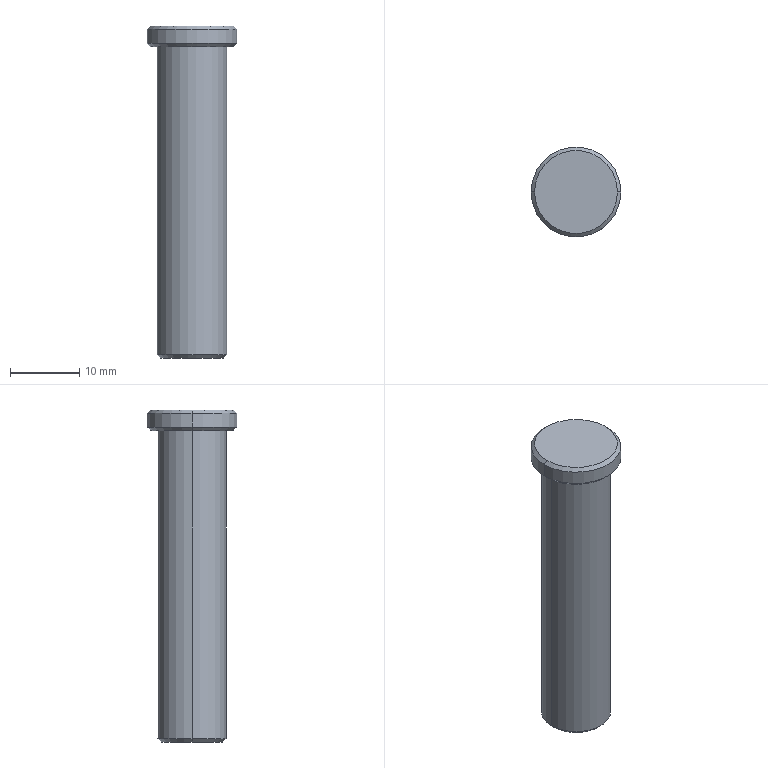Part | SolidWorks | features Chamfer 1, Extrusion 1, ICE 1 | 1 solid | 13 faces | box 13 x 13 x 48 mm | volume 3919 mm3 | cone 6 | cylinder 4 | plane 3 | commonest cylinder face diameters 10 x2 13 x2
STEP:
#1=CARTESIAN_POINT('',(-4.5,0.,0.));
#2=VERTEX_POINT('',#1);
#3=CARTESIAN_POINT('',(4.5,0.,0.));
#4=VERTEX_POINT('',#3);
#5=CARTESIAN_POINT('',(0.,0.,0.));
#6=DIRECTION('',(0.,0.,-1.));
#7=DIRECTION('',(1.,0.,0.));
#8=AXIS2_PLACEMENT_3D('',#5,#6,#7);
#9=CIRCLE('',#8,4.5);
#10=EDGE_CURVE('',#2,#4,#9,.T.);
#11=ORIENTED_EDGE('',*,*,#10,.F.);
#12=CARTESIAN_POINT('',(-5.,0.,0.5));
#13=VERTEX_POINT('',#12);
#14=CARTESIAN_POINT('',(-5.,0.,0.5));
#15=DIRECTION('',(-0.7071,0.,0.7071));
#16=VECTOR('',#15,1000.);
#17=LINE('',#14,#16);
#18=EDGE_CURVE('',#2,#13,#17,.T.);
#19=ORIENTED_EDGE('',*,*,#18,.T.);
#20=CARTESIAN_POINT('',(5.,0.,0.5));
#21=VERTEX_POINT('',#20);
#22=CARTESIAN_POINT('',(0.,0.,0.5));
#23=DIRECTION('',(0.,0.,1.));
#24=DIRECTION('',(1.,0.,0.));
#25=AXIS2_PLACEMENT_3D('',#22,#23,#24);
#26=CIRCLE('',#25,5.);
#27=EDGE_CURVE('',#21,#13,#26,.T.);
#28=ORIENTED_EDGE('',*,*,#27,.F.);
#29=CARTESIAN_POINT('',(5.,0.,0.5));
#30=DIRECTION('',(0.7071,0.,0.7071));
#31=VECTOR('',#30,1000.);
#32=LINE('',#29,#31);
#33=EDGE_CURVE('',#4,#21,#32,.T.);
#34=ORIENTED_EDGE('',*,*,#33,.F.);
#35=EDGE_LOOP('',(#11,#19,#28,#34));
#36=FACE_OUTER_BOUND('',#35,.T.);
#37=CARTESIAN_POINT('',(0.,0.,0.5));
#38=DIRECTION('',(0.,0.,1.));
#39=DIRECTION('',(1.,0.,0.));
#40=AXIS2_PLACEMENT_3D('',#37,#38,#39);
#41=CONICAL_SURFACE('',#40,5.,0.7854);
#42=ADVANCED_FACE('',(#36),#41,.T.);
#43=CARTESIAN_POINT('',(-6.,0.,45.));
#44=VERTEX_POINT('',#43);
#45=CARTESIAN_POINT('',(6.,0.,45.));
#46=VERTEX_POINT('',#45);
#47=CARTESIAN_POINT('',(0.,0.,45.));
#48=DIRECTION('',(0.,0.,-1.));
#49=DIRECTION('',(1.,0.,0.));
#50=AXIS2_PLACEMENT_3D('',#47,#48,#49);
#51=CIRCLE('',#50,6.);
#52=EDGE_CURVE('',#44,#46,#51,.T.);
#53=ORIENTED_EDGE('',*,*,#52,.F.);
#54=CARTESIAN_POINT('',(-6.5,0.,45.5));
#55=VERTEX_POINT('',#54);
#56=CARTESIAN_POINT('',(-6.5,0.,45.5));
#57=DIRECTION('',(-0.7071,0.,0.7071));
#58=VECTOR('',#57,1000.);
#59=LINE('',#56,#58);
#60=EDGE_CURVE('',#44,#55,#59,.T.);
#61=ORIENTED_EDGE('',*,*,#60,.T.);
#62=CARTESIAN_POINT('',(6.5,0.,45.5));
#63=VERTEX_POINT('',#62);
#64=CARTESIAN_POINT('',(0.,0.,45.5));
#65=DIRECTION('',(0.,0.,1.));
#66=DIRECTION('',(1.,0.,0.));
#67=AXIS2_PLACEMENT_3D('',#64,#65,#66);
#68=CIRCLE('',#67,6.5);
#69=EDGE_CURVE('',#63,#55,#68,.T.);
#70=ORIENTED_EDGE('',*,*,#69,.F.);
#71=CARTESIAN_POINT('',(6.5,0.,45.5));
#72=DIRECTION('',(0.7071,0.,0.7071));
#73=VECTOR('',#72,1000.);
#74=LINE('',#71,#73);
#75=EDGE_CURVE('',#46,#63,#74,.T.);
#76=ORIENTED_EDGE('',*,*,#75,.F.);
#77=EDGE_LOOP('',(#53,#61,#70,#76));
#78=FACE_OUTER_BOUND('',#77,.T.);
#79=CARTESIAN_POINT('',(0.,0.,45.5));
#80=DIRECTION('',(0.,0.,1.));
#81=DIRECTION('',(1.,0.,0.));
#82=AXIS2_PLACEMENT_3D('',#79,#80,#81);
#83=CONICAL_SURFACE('',#82,6.5,0.7854);
#84=ADVANCED_FACE('',(#78),#83,.T.);
#85=CARTESIAN_POINT('',(6.,0.,48.));
#86=VERTEX_POINT('',#85);
#87=CARTESIAN_POINT('',(-6.,0.,48.));
#88=VERTEX_POINT('',#87);
#89=CARTESIAN_POINT('',(0.,0.,48.));
#90=DIRECTION('',(0.,0.,1.));
#91=DIRECTION('',(1.,0.,0.));
#92=AXIS2_PLACEMENT_3D('',#89,#90,#91);
#93=CIRCLE('',#92,6.);
#94=EDGE_CURVE('',#86,#88,#93,.T.);
#95=ORIENTED_EDGE('',*,*,#94,.F.);
#96=CARTESIAN_POINT('',(6.5,0.,47.5));
#97=VERTEX_POINT('',#96);
#98=CARTESIAN_POINT('',(6.,0.,48.));
#99=DIRECTION('',(0.7071,0.,-0.7071));
#100=VECTOR('',#99,1000.);
#101=LINE('',#98,#100);
#102=EDGE_CURVE('',#86,#97,#101,.T.);
#103=ORIENTED_EDGE('',*,*,#102,.T.);
#104=CARTESIAN_POINT('',(-6.5,0.,47.5));
#105=VERTEX_POINT('',#104);
#106=CARTESIAN_POINT('',(0.,0.,47.5));
#107=DIRECTION('',(0.,0.,-1.));
#108=DIRECTION('',(1.,0.,0.));
#109=AXIS2_PLACEMENT_3D('',#106,#107,#108);
#110=CIRCLE('',#109,6.5);
#111=EDGE_CURVE('',#105,#97,#110,.T.);
#112=ORIENTED_EDGE('',*,*,#111,.F.);
#113=CARTESIAN_POINT('',(-6.,0.,48.));
#114=DIRECTION('',(-0.7071,0.,-0.7071));
#115=VECTOR('',#114,1000.);
#116=LINE('',#113,#115);
#117=EDGE_CURVE('',#88,#105,#116,.T.);
#118=ORIENTED_EDGE('',*,*,#117,.F.);
#119=EDGE_LOOP('',(#95,#103,#112,#118));
#120=FACE_OUTER_BOUND('',#119,.T.);
#121=CARTESIAN_POINT('',(0.,0.,48.));
#122=DIRECTION('',(0.,0.,-1.));
#123=DIRECTION('',(-1.,0.,0.));
#124=AXIS2_PLACEMENT_3D('',#121,#122,#123);
#125=CONICAL_SURFACE('',#124,6.,0.7854);
#126=ADVANCED_FACE('',(#120),#125,.T.);
#127=ORIENTED_EDGE('',*,*,#111,.T.);
#128=CARTESIAN_POINT('',(6.5,0.,48.));
#129=DIRECTION('',(0.,0.,-1.));
#130=VECTOR('',#129,1000.);
#131=LINE('',#128,#130);
#132=EDGE_CURVE('',#97,#63,#131,.T.);
#133=ORIENTED_EDGE('',*,*,#132,.T.);
#134=ORIENTED_EDGE('',*,*,#69,.T.);
#135=CARTESIAN_POINT('',(-6.5,0.,48.));
#136=DIRECTION('',(0.,0.,-1.));
#137=VECTOR('',#136,1000.);
#138=LINE('',#135,#137);
#139=EDGE_CURVE('',#105,#55,#138,.T.);
#140=ORIENTED_EDGE('',*,*,#139,.F.);
#141=EDGE_LOOP('',(#127,#133,#134,#140));
#142=FACE_OUTER_BOUND('',#141,.T.);
#143=CARTESIAN_POINT('',(0.,0.,48.));
#144=DIRECTION('',(0.,0.,-1.));
#145=DIRECTION('',(-1.,0.,0.));
#146=AXIS2_PLACEMENT_3D('',#143,#144,#145);
#147=CYLINDRICAL_SURFACE('',#146,6.5);
#148=ADVANCED_FACE('',(#142),#147,.T.);
#149=CARTESIAN_POINT('',(5.,0.,45.));
#150=VERTEX_POINT('',#149);
#151=CARTESIAN_POINT('',(-5.,0.,45.));
#152=VERTEX_POINT('',#151);
#153=CARTESIAN_POINT('',(0.,0.,45.));
#154=DIRECTION('',(0.,0.,1.));
#155=DIRECTION('',(1.,0.,0.));
#156=AXIS2_PLACEMENT_3D('',#153,#154,#155);
#157=CIRCLE('',#156,5.);
#158=EDGE_CURVE('',#150,#152,#157,.T.);
#159=ORIENTED_EDGE('',*,*,#158,.F.);
#160=CARTESIAN_POINT('',(5.,0.,45.));
#161=DIRECTION('',(0.,0.,-1.));
#162=VECTOR('',#161,1000.);
#163=LINE('',#160,#162);
#164=EDGE_CURVE('',#150,#21,#163,.T.);
#165=ORIENTED_EDGE('',*,*,#164,.T.);
#166=ORIENTED_EDGE('',*,*,#27,.T.);
#167=CARTESIAN_POINT('',(-5.,0.,45.));
#168=DIRECTION('',(0.,0.,-1.));
#169=VECTOR('',#168,1000.);
#170=LINE('',#167,#169);
#171=EDGE_CURVE('',#152,#13,#170,.T.);
#172=ORIENTED_EDGE('',*,*,#171,.F.);
#173=EDGE_LOOP('',(#159,#165,#166,#172));
#174=FACE_OUTER_BOUND('',#173,.T.);
#175=CARTESIAN_POINT('',(0.,0.,45.));
#176=DIRECTION('',(0.,0.,-1.));
#177=DIRECTION('',(-1.,0.,0.));
#178=AXIS2_PLACEMENT_3D('',#175,#176,#177);
#179=CYLINDRICAL_SURFACE('',#178,5.);
#180=ADVANCED_FACE('',(#174),#179,.T.);
#181=ORIENTED_EDGE('',*,*,#164,.F.);
#182=CARTESIAN_POINT('',(0.,0.,45.));
#183=DIRECTION('',(0.,0.,1.));
#184=DIRECTION('',(1.,0.,0.));
#185=AXIS2_PLACEMENT_3D('',#182,#183,#184);
#186=CIRCLE('',#185,5.);
#187=EDGE_CURVE('',#152,#150,#186,.T.);
#188=ORIENTED_EDGE('',*,*,#187,.F.);
#189=ORIENTED_EDGE('',*,*,#171,.T.);
#190=CARTESIAN_POINT('',(0.,0.,0.5));
#191=DIRECTION('',(0.,0.,1.));
#192=DIRECTION('',(1.,0.,0.));
#193=AXIS2_PLACEMENT_3D('',#190,#191,#192);
#194=CIRCLE('',#193,5.);
#195=EDGE_CURVE('',#13,#21,#194,.T.);
#196=ORIENTED_EDGE('',*,*,#195,.T.);
#197=EDGE_LOOP('',(#181,#188,#189,#196));
#198=FACE_OUTER_BOUND('',#197,.T.);
#199=CARTESIAN_POINT('',(0.,0.,45.));
#200=DIRECTION('',(0.,0.,-1.));
#201=DIRECTION('',(-1.,0.,0.));
#202=AXIS2_PLACEMENT_3D('',#199,#200,#201);
#203=CYLINDRICAL_SURFACE('',#202,5.);
#204=ADVANCED_FACE('',(#198),#203,.T.);
#205=CARTESIAN_POINT('',(0.,0.,0.));
#206=DIRECTION('',(0.,0.,-1.));
#207=DIRECTION('',(1.,0.,0.));
#208=AXIS2_PLACEMENT_3D('',#205,#206,#207);
#209=CIRCLE('',#208,4.5);
#210=EDGE_CURVE('',#4,#2,#209,.T.);
#211=ORIENTED_EDGE('',*,*,#210,.T.);
#212=ORIENTED_EDGE('',*,*,#10,.T.);
#213=EDGE_LOOP('',(#211,#212));
#214=FACE_OUTER_BOUND('',#213,.T.);
#215=CARTESIAN_POINT('',(0.,0.,0.));
#216=DIRECTION('',(0.,0.,1.));
#217=DIRECTION('',(1.,0.,0.));
#218=AXIS2_PLACEMENT_3D('',#215,#216,#217);
#219=PLANE('',#218);
#220=ADVANCED_FACE('',(#214),#219,.F.);
#221=ORIENTED_EDGE('',*,*,#132,.F.);
#222=CARTESIAN_POINT('',(0.,0.,47.5));
#223=DIRECTION('',(0.,0.,-1.));
#224=DIRECTION('',(1.,0.,0.));
#225=AXIS2_PLACEMENT_3D('',#222,#223,#224);
#226=CIRCLE('',#225,6.5);
#227=EDGE_CURVE('',#97,#105,#226,.T.);
#228=ORIENTED_EDGE('',*,*,#227,.T.);
#229=ORIENTED_EDGE('',*,*,#139,.T.);
#230=CARTESIAN_POINT('',(0.,0.,45.5));
#231=DIRECTION('',(0.,0.,1.));
#232=DIRECTION('',(1.,0.,0.));
#233=AXIS2_PLACEMENT_3D('',#230,#231,#232);
#234=CIRCLE('',#233,6.5);
#235=EDGE_CURVE('',#55,#63,#234,.T.);
#236=ORIENTED_EDGE('',*,*,#235,.T.);
#237=EDGE_LOOP('',(#221,#228,#229,#236));
#238=FACE_OUTER_BOUND('',#237,.T.);
#239=CARTESIAN_POINT('',(0.,0.,48.));
#240=DIRECTION('',(0.,0.,-1.));
#241=DIRECTION('',(-1.,0.,0.));
#242=AXIS2_PLACEMENT_3D('',#239,#240,#241);
#243=CYLINDRICAL_SURFACE('',#242,6.5);
#244=ADVANCED_FACE('',(#238),#243,.T.);
#245=CARTESIAN_POINT('',(0.,0.,48.));
#246=DIRECTION('',(0.,0.,1.));
#247=DIRECTION('',(1.,0.,0.));
#248=AXIS2_PLACEMENT_3D('',#245,#246,#247);
#249=CIRCLE('',#248,6.);
#250=EDGE_CURVE('',#88,#86,#249,.T.);
#251=ORIENTED_EDGE('',*,*,#250,.T.);
#252=ORIENTED_EDGE('',*,*,#94,.T.);
#253=EDGE_LOOP('',(#251,#252));
#254=FACE_OUTER_BOUND('',#253,.T.);
#255=CARTESIAN_POINT('',(0.,0.,48.));
#256=DIRECTION('',(0.,0.,1.));
#257=DIRECTION('',(1.,0.,0.));
#258=AXIS2_PLACEMENT_3D('',#255,#256,#257);
#259=PLANE('',#258);
#260=ADVANCED_FACE('',(#254),#259,.T.);
#261=CARTESIAN_POINT('',(0.,0.,45.));
#262=DIRECTION('',(0.,0.,-1.));
#263=DIRECTION('',(1.,0.,0.));
#264=AXIS2_PLACEMENT_3D('',#261,#262,#263);
#265=CIRCLE('',#264,6.);
#266=EDGE_CURVE('',#46,#44,#265,.T.);
#267=ORIENTED_EDGE('',*,*,#266,.T.);
#268=ORIENTED_EDGE('',*,*,#52,.T.);
#269=EDGE_LOOP('',(#267,#268));
#270=FACE_OUTER_BOUND('',#269,.T.);
#271=ORIENTED_EDGE('',*,*,#187,.T.);
#272=ORIENTED_EDGE('',*,*,#158,.T.);
#273=EDGE_LOOP('',(#271,#272));
#274=FACE_BOUND('',#273,.T.);
#275=CARTESIAN_POINT('',(0.,0.,45.));
#276=DIRECTION('',(0.,0.,1.));
#277=DIRECTION('',(1.,0.,0.));
#278=AXIS2_PLACEMENT_3D('',#275,#276,#277);
#279=PLANE('',#278);
#280=ADVANCED_FACE('',(#270,#274),#279,.F.);
#281=ORIENTED_EDGE('',*,*,#102,.F.);
#282=ORIENTED_EDGE('',*,*,#250,.F.);
#283=ORIENTED_EDGE('',*,*,#117,.T.);
#284=ORIENTED_EDGE('',*,*,#227,.F.);
#285=EDGE_LOOP('',(#281,#282,#283,#284));
#286=FACE_OUTER_BOUND('',#285,.T.);
#287=CARTESIAN_POINT('',(0.,0.,48.));
#288=DIRECTION('',(0.,0.,-1.));
#289=DIRECTION('',(-1.,0.,0.));
#290=AXIS2_PLACEMENT_3D('',#287,#288,#289);
#291=CONICAL_SURFACE('',#290,6.,0.7854);
#292=ADVANCED_FACE('',(#286),#291,.T.);
#293=ORIENTED_EDGE('',*,*,#60,.F.);
#294=ORIENTED_EDGE('',*,*,#266,.F.);
#295=ORIENTED_EDGE('',*,*,#75,.T.);
#296=ORIENTED_EDGE('',*,*,#235,.F.);
#297=EDGE_LOOP('',(#293,#294,#295,#296));
#298=FACE_OUTER_BOUND('',#297,.T.);
#299=CARTESIAN_POINT('',(0.,0.,45.5));
#300=DIRECTION('',(0.,0.,1.));
#301=DIRECTION('',(1.,0.,0.));
#302=AXIS2_PLACEMENT_3D('',#299,#300,#301);
#303=CONICAL_SURFACE('',#302,6.5,0.7854);
#304=ADVANCED_FACE('',(#298),#303,.T.);
#305=ORIENTED_EDGE('',*,*,#18,.F.);
#306=ORIENTED_EDGE('',*,*,#210,.F.);
#307=ORIENTED_EDGE('',*,*,#33,.T.);
#308=ORIENTED_EDGE('',*,*,#195,.F.);
#309=EDGE_LOOP('',(#305,#306,#307,#308));
#310=FACE_OUTER_BOUND('',#309,.T.);
#311=CARTESIAN_POINT('',(0.,0.,0.5));
#312=DIRECTION('',(0.,0.,1.));
#313=DIRECTION('',(1.,0.,0.));
#314=AXIS2_PLACEMENT_3D('',#311,#312,#313);
#315=CONICAL_SURFACE('',#314,5.,0.7854);
#316=ADVANCED_FACE('',(#310),#315,.T.);
#317=CLOSED_SHELL('',(#42,#84,#126,#148,#180,#204,#220,#244,#260,#280,#292,#304,#316));
#318=MANIFOLD_SOLID_BREP('',#317);
#319=CARTESIAN_POINT('',(0.,0.,0.));
#320=DIRECTION('',(0.,0.,1.));
#321=DIRECTION('',(1.,0.,0.));
#322=AXIS2_PLACEMENT_3D('',#319,#320,#321);
#323=(LENGTH_UNIT()NAMED_UNIT(*)SI_UNIT(.MILLI.,.METRE.));
#324=UNCERTAINTY_MEASURE_WITH_UNIT(LENGTH_MEASURE(0.00001),#323,'','');
#325=(NAMED_UNIT(*)PLANE_ANGLE_UNIT()SI_UNIT($,.RADIAN.));
#326=(NAMED_UNIT(*)SI_UNIT($,.STERADIAN.)SOLID_ANGLE_UNIT());
#327=(GEOMETRIC_REPRESENTATION_CONTEXT(3)GLOBAL_UNCERTAINTY_ASSIGNED_CONTEXT((#324))GLOBAL_UNIT_ASSIGNED_CONTEXT((#323,#325,#326))REPRESENTATION_CONTEXT('',''));
#328=ADVANCED_BREP_SHAPE_REPRESENTATION('',(#318,#322),#327);